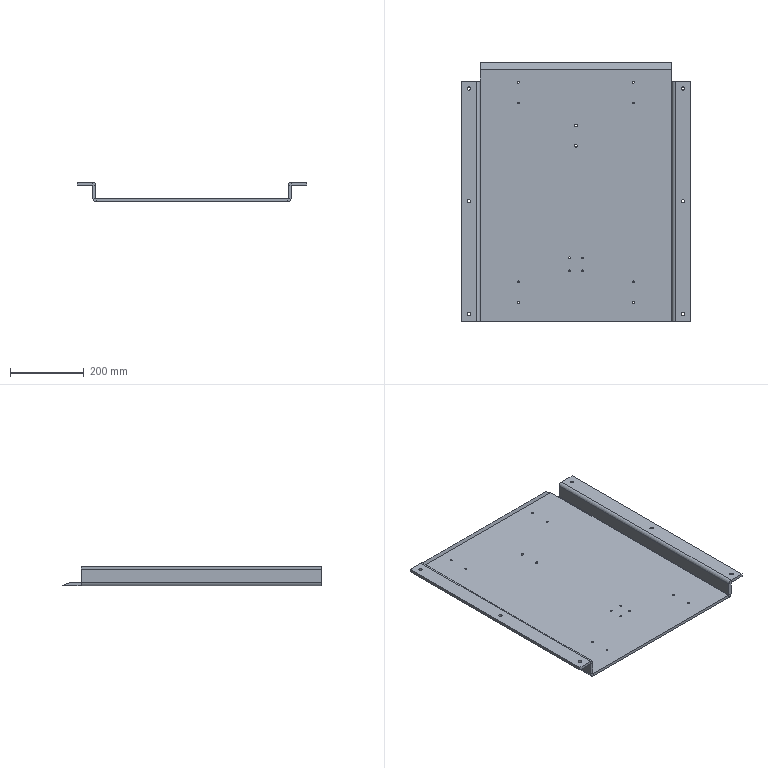Part | STEP file | X77-03302 | 1 solid | 79 faces | box 620 x 700 x 53 mm | volume 3816269 mm3 | cylinder 48 | plane 31 | commonest cylinder face diameters 5 x16 9 x12 4.2 x8 1.473 x4 6.8 x4 17.473 x4